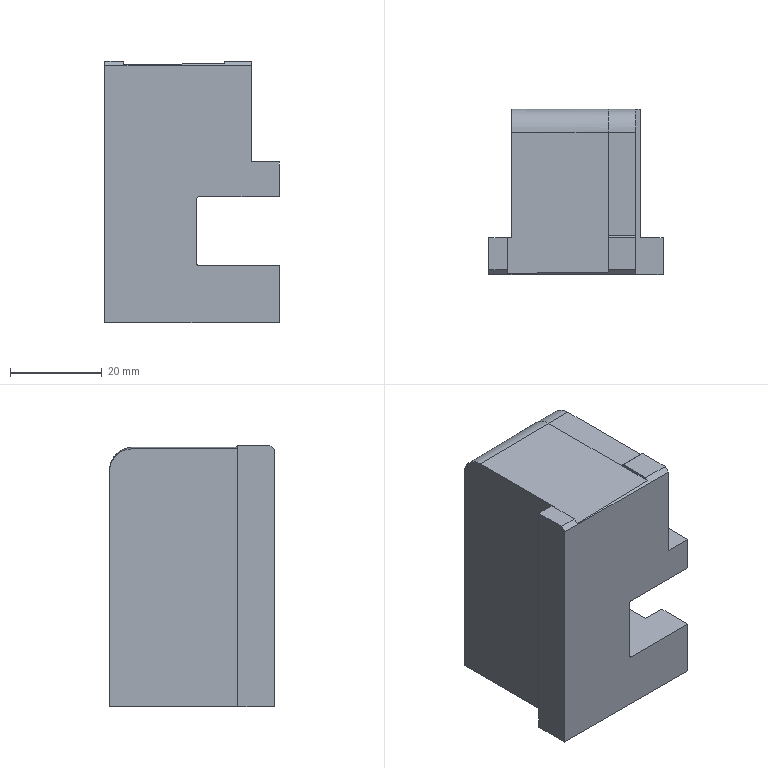Part | STEP file | dao nhan khong logo | 1 solid | 38 faces | box 38 x 36 x 57.1 mm | volume 51330 mm3 | plane 27 | cylinder 7 | cone 4 | commonest cylinder face diameters 1 x3 8.376 x2 10 x2